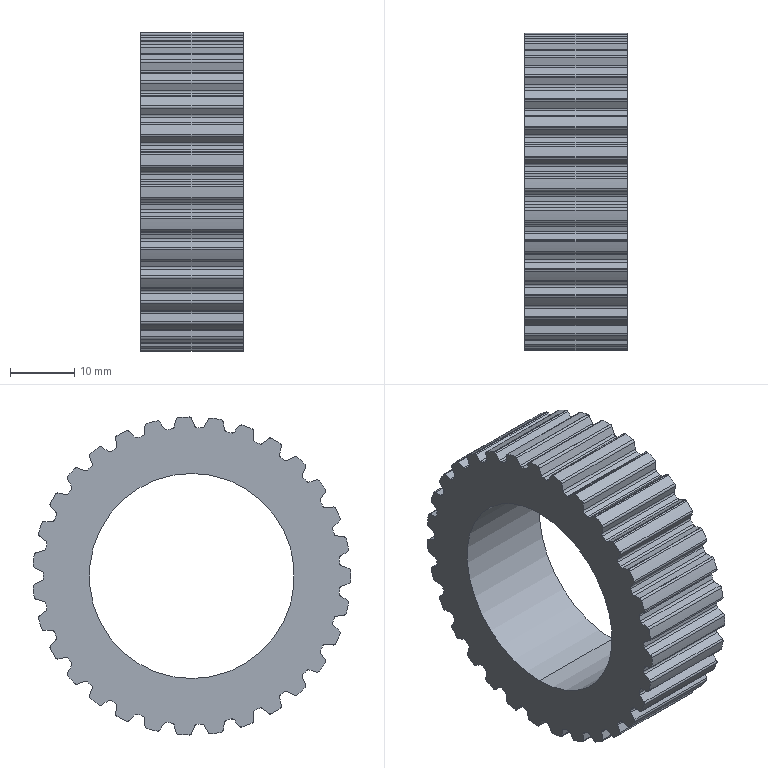Part | SolidWorks | features CirPattern 1, Cut 1, ICE 1, RefAxis 1, Revolution 1 | 1 solid | 275 faces | box 16 x 49.566 x 49.615 mm | volume 16375 mm3 | cylinder 211 | plane 64 | commonest cylinder face diameters 0.76 x74 0.82 x73 46.322 x31 49.622 x31 32 x2